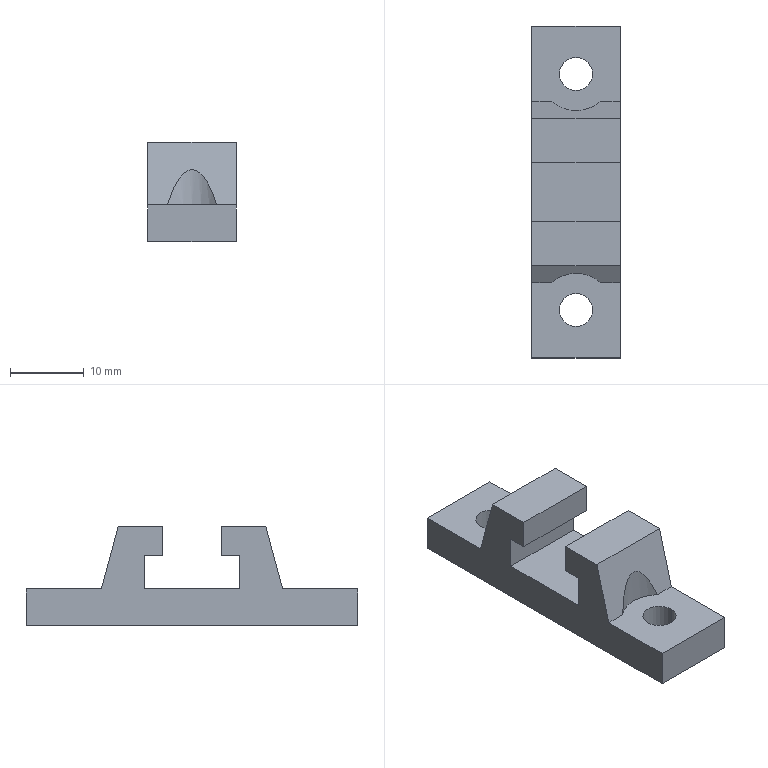Part | STEP file | hlre7_2_03 | 1 solid | 24 faces | box 12 x 45 x 13.5 mm | volume 3705 mm3 | plane 18 | cylinder 6 | commonest cylinder face diameters 4.5 x4 10 x2